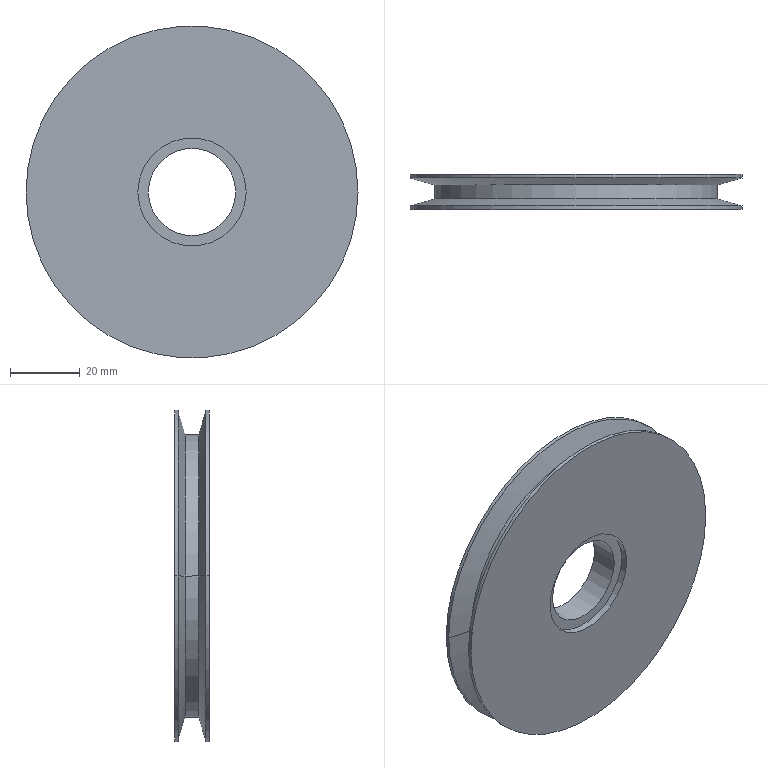Part | STEP file | BCC3 H16_2 | 1 solid | 17 faces | box 95 x 10 x 95 mm | volume 53732 mm3 | cylinder 10 | cone 4 | plane 3 | commonest cylinder face diameters 95 x4 25 x2 31 x2 81 x2
STEP:
#1=CARTESIAN_POINT('',(0.,0.,0.));
#2=DIRECTION('',(0.,0.,1.));
#3=DIRECTION('',(1.,0.,0.));
#4=AXIS2_PLACEMENT_3D('',#1,#2,#3);
#5=CARTESIAN_POINT('',(15.5,2.,0.));
#6=VERTEX_POINT('',#5);
#7=CARTESIAN_POINT('',(15.5,0.,0.));
#8=VERTEX_POINT('',#7);
#9=CARTESIAN_POINT('',(15.5,2.,0.));
#10=DIRECTION('',(0.,-1.,0.));
#11=VECTOR('',#10,1.);
#12=LINE('',#9,#11);
#13=CARTESIAN_POINT('',(0.,2.,0.));
#14=DIRECTION('',(0.,-1.,0.));
#15=DIRECTION('',(1.,0.,0.));
#16=AXIS2_PLACEMENT_3D('',#13,#14,#15);
#17=CYLINDRICAL_SURFACE('',#16,15.5);
#18=CARTESIAN_POINT('',(6.283,0.));
#19=DIRECTION('',(0.,1.));
#20=VECTOR('',#19,1.);
#21=LINE('',#18,#20);
#22=(GEOMETRIC_REPRESENTATION_CONTEXT(2)PARAMETRIC_REPRESENTATION_CONTEXT()REPRESENTATION_CONTEXT('',''));
#23=DEFINITIONAL_REPRESENTATION('',(#21),#22);
#24=PCURVE('',#17,#23);
#25=CARTESIAN_POINT('',(0.,2.,0.));
#26=DIRECTION('',(0.,-1.,0.));
#27=DIRECTION('',(1.,0.,0.));
#28=AXIS2_PLACEMENT_3D('',#25,#26,#27);
#29=CYLINDRICAL_SURFACE('',#28,15.5);
#30=CARTESIAN_POINT('',(0.,0.));
#31=DIRECTION('',(0.,1.));
#32=VECTOR('',#31,1.);
#33=LINE('',#30,#32);
#34=(GEOMETRIC_REPRESENTATION_CONTEXT(2)PARAMETRIC_REPRESENTATION_CONTEXT()REPRESENTATION_CONTEXT('',''));
#35=DEFINITIONAL_REPRESENTATION('',(#33),#34);
#36=PCURVE('',#29,#35);
#37=SURFACE_CURVE('',#12,(#24,#36),.PCURVE_S1.);
#38=EDGE_CURVE('',#6,#8,#37,.T.);
#39=ORIENTED_EDGE('',*,*,#38,.T.);
#40=CARTESIAN_POINT('',(-15.5,0.,0.));
#41=VERTEX_POINT('',#40);
#42=CARTESIAN_POINT('',(0.,0.,0.));
#43=DIRECTION('',(0.,1.,0.));
#44=DIRECTION('',(-1.,0.,0.));
#45=AXIS2_PLACEMENT_3D('',#42,#43,#44);
#46=CIRCLE('',#45,15.5);
#47=CARTESIAN_POINT('',(9.425,2.));
#48=DIRECTION('',(-1.,0.));
#49=VECTOR('',#48,1.);
#50=LINE('',#47,#49);
#51=(GEOMETRIC_REPRESENTATION_CONTEXT(2)PARAMETRIC_REPRESENTATION_CONTEXT()REPRESENTATION_CONTEXT('',''));
#52=DEFINITIONAL_REPRESENTATION('',(#50),#51);
#53=PCURVE('',#17,#52);
#54=CARTESIAN_POINT('',(47.5,0.,0.));
#55=DIRECTION('',(0.,-1.,0.));
#56=DIRECTION('',(1.,0.,0.));
#57=AXIS2_PLACEMENT_3D('',#54,#55,#56);
#58=PLANE('',#57);
#59=CARTESIAN_POINT('',(-63.,0.));
#60=CARTESIAN_POINT('',(-63.,26.847));
#61=CARTESIAN_POINT('',(-39.75,13.423));
#62=CARTESIAN_POINT('',(-16.5,0.));
#63=CARTESIAN_POINT('',(-39.75,-13.423));
#64=CARTESIAN_POINT('',(-63.,-26.847));
#65=CARTESIAN_POINT('',(-63.,0.));
#66=(BOUNDED_CURVE()B_SPLINE_CURVE(2,(#59,#60,#61,#62,#63,#64,#65),.UNSPECIFIED.,.T.,.F.)B_SPLINE_CURVE_WITH_KNOTS((1,2,2,2,2,1),(-2.094,0.,2.094,4.189,6.283,8.378),.UNSPECIFIED.)CURVE()GEOMETRIC_REPRESENTATION_ITEM()RATIONAL_B_SPLINE_CURVE((1.,0.5,1.,0.5,1.,0.5,1.))REPRESENTATION_ITEM(''));
#67=(GEOMETRIC_REPRESENTATION_CONTEXT(2)PARAMETRIC_REPRESENTATION_CONTEXT()REPRESENTATION_CONTEXT('',''));
#68=DEFINITIONAL_REPRESENTATION('',(#66),#67);
#69=PCURVE('',#58,#68);
#70=SURFACE_CURVE('',#46,(#53,#69),.PCURVE_S1.);
#71=EDGE_CURVE('',#8,#41,#70,.T.);
#72=ORIENTED_EDGE('',*,*,#71,.T.);
#73=CARTESIAN_POINT('',(-15.5,2.,0.));
#74=VERTEX_POINT('',#73);
#75=CARTESIAN_POINT('',(-15.5,2.,0.));
#76=DIRECTION('',(0.,-1.,0.));
#77=VECTOR('',#76,1.);
#78=LINE('',#75,#77);
#79=CARTESIAN_POINT('',(3.142,0.));
#80=DIRECTION('',(0.,1.));
#81=VECTOR('',#80,1.);
#82=LINE('',#79,#81);
#83=(GEOMETRIC_REPRESENTATION_CONTEXT(2)PARAMETRIC_REPRESENTATION_CONTEXT()REPRESENTATION_CONTEXT('',''));
#84=DEFINITIONAL_REPRESENTATION('',(#82),#83);
#85=PCURVE('',#17,#84);
#86=CARTESIAN_POINT('',(3.142,0.));
#87=DIRECTION('',(0.,1.));
#88=VECTOR('',#87,1.);
#89=LINE('',#86,#88);
#90=(GEOMETRIC_REPRESENTATION_CONTEXT(2)PARAMETRIC_REPRESENTATION_CONTEXT()REPRESENTATION_CONTEXT('',''));
#91=DEFINITIONAL_REPRESENTATION('',(#89),#90);
#92=PCURVE('',#29,#91);
#93=SURFACE_CURVE('',#78,(#85,#92),.PCURVE_S1.);
#94=EDGE_CURVE('',#74,#41,#93,.T.);
#95=ORIENTED_EDGE('',*,*,#94,.F.);
#96=CARTESIAN_POINT('',(0.,2.,0.));
#97=DIRECTION('',(0.,1.,0.));
#98=DIRECTION('',(-1.,0.,0.));
#99=AXIS2_PLACEMENT_3D('',#96,#97,#98);
#100=CIRCLE('',#99,15.5);
#101=CARTESIAN_POINT('',(9.425,0.));
#102=DIRECTION('',(-1.,0.));
#103=VECTOR('',#102,1.);
#104=LINE('',#101,#103);
#105=(GEOMETRIC_REPRESENTATION_CONTEXT(2)PARAMETRIC_REPRESENTATION_CONTEXT()REPRESENTATION_CONTEXT('',''));
#106=DEFINITIONAL_REPRESENTATION('',(#104),#105);
#107=PCURVE('',#17,#106);
#108=CARTESIAN_POINT('',(0.,2.,0.));
#109=DIRECTION('',(0.,1.,0.));
#110=DIRECTION('',(-1.,0.,0.));
#111=AXIS2_PLACEMENT_3D('',#108,#109,#110);
#112=PLANE('',#111);
#113=CARTESIAN_POINT('',(0.,0.));
#114=DIRECTION('',(1.,0.));
#115=AXIS2_PLACEMENT_2D('',#113,#114);
#116=CIRCLE('',#115,15.5);
#117=(GEOMETRIC_REPRESENTATION_CONTEXT(2)PARAMETRIC_REPRESENTATION_CONTEXT()REPRESENTATION_CONTEXT('',''));
#118=DEFINITIONAL_REPRESENTATION('',(#116),#117);
#119=PCURVE('',#112,#118);
#120=SURFACE_CURVE('',#100,(#107,#119),.PCURVE_S1.);
#121=EDGE_CURVE('',#6,#74,#120,.T.);
#122=ORIENTED_EDGE('',*,*,#121,.F.);
#123=EDGE_LOOP('',(#39,#72,#95,#122));
#124=FACE_BOUND('',#123,.F.);
#125=ADVANCED_FACE('',(#124),#17,.F.);
#126=CARTESIAN_POINT('',(12.5,10.,0.));
#127=VERTEX_POINT('',#126);
#128=CARTESIAN_POINT('',(12.5,2.,0.));
#129=VERTEX_POINT('',#128);
#130=CARTESIAN_POINT('',(12.5,0.,0.));
#131=DIRECTION('',(0.,-1.,0.));
#132=VECTOR('',#131,1.);
#133=LINE('',#130,#132);
#134=CARTESIAN_POINT('',(0.,0.,0.));
#135=DIRECTION('',(0.,-1.,0.));
#136=DIRECTION('',(1.,0.,0.));
#137=AXIS2_PLACEMENT_3D('',#134,#135,#136);
#138=CYLINDRICAL_SURFACE('',#137,12.5);
#139=CARTESIAN_POINT('',(6.283,0.));
#140=DIRECTION('',(0.,1.));
#141=VECTOR('',#140,1.);
#142=LINE('',#139,#141);
#143=(GEOMETRIC_REPRESENTATION_CONTEXT(2)PARAMETRIC_REPRESENTATION_CONTEXT()REPRESENTATION_CONTEXT('',''));
#144=DEFINITIONAL_REPRESENTATION('',(#142),#143);
#145=PCURVE('',#138,#144);
#146=CARTESIAN_POINT('',(0.,0.,0.));
#147=DIRECTION('',(0.,-1.,0.));
#148=DIRECTION('',(1.,0.,0.));
#149=AXIS2_PLACEMENT_3D('',#146,#147,#148);
#150=CYLINDRICAL_SURFACE('',#149,12.5);
#151=CARTESIAN_POINT('',(0.,0.));
#152=DIRECTION('',(0.,1.));
#153=VECTOR('',#152,1.);
#154=LINE('',#151,#153);
#155=(GEOMETRIC_REPRESENTATION_CONTEXT(2)PARAMETRIC_REPRESENTATION_CONTEXT()REPRESENTATION_CONTEXT('',''));
#156=DEFINITIONAL_REPRESENTATION('',(#154),#155);
#157=PCURVE('',#150,#156);
#158=SURFACE_CURVE('',#133,(#145,#157),.PCURVE_S1.);
#159=EDGE_CURVE('',#127,#129,#158,.T.);
#160=ORIENTED_EDGE('',*,*,#159,.T.);
#161=CARTESIAN_POINT('',(-12.5,2.,0.));
#162=VERTEX_POINT('',#161);
#163=CARTESIAN_POINT('',(0.,2.,0.));
#164=DIRECTION('',(0.,1.,0.));
#165=DIRECTION('',(-1.,0.,0.));
#166=AXIS2_PLACEMENT_3D('',#163,#164,#165);
#167=CIRCLE('',#166,12.5);
#168=CARTESIAN_POINT('',(9.425,-2.));
#169=DIRECTION('',(-1.,0.));
#170=VECTOR('',#169,1.);
#171=LINE('',#168,#170);
#172=(GEOMETRIC_REPRESENTATION_CONTEXT(2)PARAMETRIC_REPRESENTATION_CONTEXT()REPRESENTATION_CONTEXT('',''));
#173=DEFINITIONAL_REPRESENTATION('',(#171),#172);
#174=PCURVE('',#138,#173);
#175=CARTESIAN_POINT('',(0.,0.));
#176=DIRECTION('',(1.,0.));
#177=AXIS2_PLACEMENT_2D('',#175,#176);
#178=CIRCLE('',#177,12.5);
#179=(GEOMETRIC_REPRESENTATION_CONTEXT(2)PARAMETRIC_REPRESENTATION_CONTEXT()REPRESENTATION_CONTEXT('',''));
#180=DEFINITIONAL_REPRESENTATION('',(#178),#179);
#181=PCURVE('',#112,#180);
#182=SURFACE_CURVE('',#167,(#174,#181),.PCURVE_S1.);
#183=EDGE_CURVE('',#129,#162,#182,.T.);
#184=ORIENTED_EDGE('',*,*,#183,.T.);
#185=CARTESIAN_POINT('',(-12.5,10.,0.));
#186=VERTEX_POINT('',#185);
#187=CARTESIAN_POINT('',(-12.5,0.,0.));
#188=DIRECTION('',(0.,-1.,0.));
#189=VECTOR('',#188,1.);
#190=LINE('',#187,#189);
#191=CARTESIAN_POINT('',(3.142,0.));
#192=DIRECTION('',(0.,1.));
#193=VECTOR('',#192,1.);
#194=LINE('',#191,#193);
#195=(GEOMETRIC_REPRESENTATION_CONTEXT(2)PARAMETRIC_REPRESENTATION_CONTEXT()REPRESENTATION_CONTEXT('',''));
#196=DEFINITIONAL_REPRESENTATION('',(#194),#195);
#197=PCURVE('',#138,#196);
#198=CARTESIAN_POINT('',(3.142,0.));
#199=DIRECTION('',(0.,1.));
#200=VECTOR('',#199,1.);
#201=LINE('',#198,#200);
#202=(GEOMETRIC_REPRESENTATION_CONTEXT(2)PARAMETRIC_REPRESENTATION_CONTEXT()REPRESENTATION_CONTEXT('',''));
#203=DEFINITIONAL_REPRESENTATION('',(#201),#202);
#204=PCURVE('',#150,#203);
#205=SURFACE_CURVE('',#190,(#197,#204),.PCURVE_S1.);
#206=EDGE_CURVE('',#186,#162,#205,.T.);
#207=ORIENTED_EDGE('',*,*,#206,.F.);
#208=CARTESIAN_POINT('',(0.,10.,0.));
#209=DIRECTION('',(0.,-1.,0.));
#210=DIRECTION('',(1.,0.,0.));
#211=AXIS2_PLACEMENT_3D('',#208,#209,#210);
#212=CIRCLE('',#211,12.5);
#213=CARTESIAN_POINT('',(0.,-10.));
#214=DIRECTION('',(1.,0.));
#215=VECTOR('',#214,1.);
#216=LINE('',#213,#215);
#217=(GEOMETRIC_REPRESENTATION_CONTEXT(2)PARAMETRIC_REPRESENTATION_CONTEXT()REPRESENTATION_CONTEXT('',''));
#218=DEFINITIONAL_REPRESENTATION('',(#216),#217);
#219=PCURVE('',#138,#218);
#220=CARTESIAN_POINT('',(12.5,10.,0.));
#221=DIRECTION('',(0.,1.,0.));
#222=DIRECTION('',(-1.,0.,0.));
#223=AXIS2_PLACEMENT_3D('',#220,#221,#222);
#224=PLANE('',#223);
#225=CARTESIAN_POINT('',(0.,0.));
#226=CARTESIAN_POINT('',(0.,21.651));
#227=CARTESIAN_POINT('',(18.75,10.825));
#228=CARTESIAN_POINT('',(37.5,0.));
#229=CARTESIAN_POINT('',(18.75,-10.825));
#230=CARTESIAN_POINT('',(0.,-21.651));
#231=CARTESIAN_POINT('',(0.,0.));
#232=(BOUNDED_CURVE()B_SPLINE_CURVE(2,(#225,#226,#227,#228,#229,#230,#231),.UNSPECIFIED.,.T.,.F.)B_SPLINE_CURVE_WITH_KNOTS((1,2,2,2,2,1),(-2.094,0.,2.094,4.189,6.283,8.378),.UNSPECIFIED.)CURVE()GEOMETRIC_REPRESENTATION_ITEM()RATIONAL_B_SPLINE_CURVE((1.,0.5,1.,0.5,1.,0.5,1.))REPRESENTATION_ITEM(''));
#233=(GEOMETRIC_REPRESENTATION_CONTEXT(2)PARAMETRIC_REPRESENTATION_CONTEXT()REPRESENTATION_CONTEXT('',''));
#234=DEFINITIONAL_REPRESENTATION('',(#232),#233);
#235=PCURVE('',#224,#234);
#236=SURFACE_CURVE('',#212,(#219,#235),.PCURVE_S1.);
#237=EDGE_CURVE('',#186,#127,#236,.T.);
#238=ORIENTED_EDGE('',*,*,#237,.T.);
#239=EDGE_LOOP('',(#160,#184,#207,#238));
#240=FACE_BOUND('',#239,.F.);
#241=ADVANCED_FACE('',(#240),#138,.F.);
#242=CARTESIAN_POINT('',(47.5,1.,0.));
#243=VERTEX_POINT('',#242);
#244=CARTESIAN_POINT('',(-47.5,1.,0.));
#245=VERTEX_POINT('',#244);
#246=CARTESIAN_POINT('',(0.,1.,0.));
#247=DIRECTION('',(0.,-1.,0.));
#248=DIRECTION('',(1.,0.,0.));
#249=AXIS2_PLACEMENT_3D('',#246,#247,#248);
#250=CIRCLE('',#249,47.5);
#251=CARTESIAN_POINT('',(0.,0.,0.));
#252=DIRECTION('',(0.,-1.,0.));
#253=DIRECTION('',(1.,0.,0.));
#254=AXIS2_PLACEMENT_3D('',#251,#252,#253);
#255=CYLINDRICAL_SURFACE('',#254,47.5);
#256=CARTESIAN_POINT('',(0.,-1.));
#257=DIRECTION('',(1.,0.));
#258=VECTOR('',#257,1.);
#259=LINE('',#256,#258);
#260=(GEOMETRIC_REPRESENTATION_CONTEXT(2)PARAMETRIC_REPRESENTATION_CONTEXT()REPRESENTATION_CONTEXT('',''));
#261=DEFINITIONAL_REPRESENTATION('',(#259),#260);
#262=PCURVE('',#255,#261);
#263=CARTESIAN_POINT('',(0.,1.,0.));
#264=DIRECTION('',(0.,-1.,0.));
#265=DIRECTION('',(1.,0.,0.));
#266=AXIS2_PLACEMENT_3D('',#263,#264,#265);
#267=CONICAL_SURFACE('',#266,47.5,1.292);
#268=CARTESIAN_POINT('',(0.,0.));
#269=DIRECTION('',(1.,0.));
#270=VECTOR('',#269,1.);
#271=LINE('',#268,#270);
#272=(GEOMETRIC_REPRESENTATION_CONTEXT(2)PARAMETRIC_REPRESENTATION_CONTEXT()REPRESENTATION_CONTEXT('',''));
#273=DEFINITIONAL_REPRESENTATION('',(#271),#272);
#274=PCURVE('',#267,#273);
#275=SURFACE_CURVE('',#250,(#262,#274),.PCURVE_S1.);
#276=EDGE_CURVE('',#243,#245,#275,.T.);
#277=ORIENTED_EDGE('',*,*,#276,.T.);
#278=CARTESIAN_POINT('',(-47.5,0.,0.));
#279=VERTEX_POINT('',#278);
#280=CARTESIAN_POINT('',(-47.5,0.,0.));
#281=DIRECTION('',(0.,-1.,0.));
#282=VECTOR('',#281,1.);
#283=LINE('',#280,#282);
#284=CARTESIAN_POINT('',(3.142,0.));
#285=DIRECTION('',(0.,1.));
#286=VECTOR('',#285,1.);
#287=LINE('',#284,#286);
#288=(GEOMETRIC_REPRESENTATION_CONTEXT(2)PARAMETRIC_REPRESENTATION_CONTEXT()REPRESENTATION_CONTEXT('',''));
#289=DEFINITIONAL_REPRESENTATION('',(#287),#288);
#290=PCURVE('',#255,#289);
#291=CARTESIAN_POINT('',(0.,0.,0.));
#292=DIRECTION('',(0.,-1.,0.));
#293=DIRECTION('',(1.,0.,0.));
#294=AXIS2_PLACEMENT_3D('',#291,#292,#293);
#295=CYLINDRICAL_SURFACE('',#294,47.5);
#296=CARTESIAN_POINT('',(3.142,0.));
#297=DIRECTION('',(0.,1.));
#298=VECTOR('',#297,1.);
#299=LINE('',#296,#298);
#300=(GEOMETRIC_REPRESENTATION_CONTEXT(2)PARAMETRIC_REPRESENTATION_CONTEXT()REPRESENTATION_CONTEXT('',''));
#301=DEFINITIONAL_REPRESENTATION('',(#299),#300);
#302=PCURVE('',#295,#301);
#303=SURFACE_CURVE('',#283,(#290,#302),.PCURVE_S1.);
#304=EDGE_CURVE('',#245,#279,#303,.T.);
#305=ORIENTED_EDGE('',*,*,#304,.T.);
#306=CARTESIAN_POINT('',(47.5,0.,0.));
#307=VERTEX_POINT('',#306);
#308=CARTESIAN_POINT('',(0.,0.,0.));
#309=DIRECTION('',(0.,-1.,0.));
#310=DIRECTION('',(1.,0.,0.));
#311=AXIS2_PLACEMENT_3D('',#308,#309,#310);
#312=CIRCLE('',#311,47.5);
#313=CARTESIAN_POINT('',(0.,0.));
#314=DIRECTION('',(1.,0.));
#315=VECTOR('',#314,1.);
#316=LINE('',#313,#315);
#317=(GEOMETRIC_REPRESENTATION_CONTEXT(2)PARAMETRIC_REPRESENTATION_CONTEXT()REPRESENTATION_CONTEXT('',''));
#318=DEFINITIONAL_REPRESENTATION('',(#316),#317);
#319=PCURVE('',#255,#318);
#320=CARTESIAN_POINT('',(-47.5,0.));
#321=DIRECTION('',(1.,0.));
#322=AXIS2_PLACEMENT_2D('',#320,#321);
#323=CIRCLE('',#322,47.5);
#324=(GEOMETRIC_REPRESENTATION_CONTEXT(2)PARAMETRIC_REPRESENTATION_CONTEXT()REPRESENTATION_CONTEXT('',''));
#325=DEFINITIONAL_REPRESENTATION('',(#323),#324);
#326=PCURVE('',#58,#325);
#327=SURFACE_CURVE('',#312,(#319,#326),.PCURVE_S1.);
#328=EDGE_CURVE('',#307,#279,#327,.T.);
#329=ORIENTED_EDGE('',*,*,#328,.F.);
#330=CARTESIAN_POINT('',(47.5,0.,0.));
#331=DIRECTION('',(0.,-1.,0.));
#332=VECTOR('',#331,1.);
#333=LINE('',#330,#332);
#334=CARTESIAN_POINT('',(0.,0.));
#335=DIRECTION('',(0.,1.));
#336=VECTOR('',#335,1.);
#337=LINE('',#334,#336);
#338=(GEOMETRIC_REPRESENTATION_CONTEXT(2)PARAMETRIC_REPRESENTATION_CONTEXT()REPRESENTATION_CONTEXT('',''));
#339=DEFINITIONAL_REPRESENTATION('',(#337),#338);
#340=PCURVE('',#255,#339);
#341=CARTESIAN_POINT('',(6.283,0.));
#342=DIRECTION('',(0.,1.));
#343=VECTOR('',#342,1.);
#344=LINE('',#341,#343);
#345=(GEOMETRIC_REPRESENTATION_CONTEXT(2)PARAMETRIC_REPRESENTATION_CONTEXT()REPRESENTATION_CONTEXT('',''));
#346=DEFINITIONAL_REPRESENTATION('',(#344),#345);
#347=PCURVE('',#295,#346);
#348=SURFACE_CURVE('',#333,(#340,#347),.PCURVE_S1.);
#349=EDGE_CURVE('',#243,#307,#348,.T.);
#350=ORIENTED_EDGE('',*,*,#349,.F.);
#351=EDGE_LOOP('',(#277,#305,#329,#350));
#352=FACE_BOUND('',#351,.T.);
#353=ADVANCED_FACE('',(#352),#255,.T.);
#354=CARTESIAN_POINT('',(40.5,3.,0.));
#355=VERTEX_POINT('',#354);
#356=CARTESIAN_POINT('',(-40.5,3.,0.));
#357=VERTEX_POINT('',#356);
#358=CARTESIAN_POINT('',(0.,3.,0.));
#359=DIRECTION('',(0.,-1.,0.));
#360=DIRECTION('',(1.,0.,0.));
#361=AXIS2_PLACEMENT_3D('',#358,#359,#360);
#362=CIRCLE('',#361,40.5);
#363=CARTESIAN_POINT('',(0.,-2.));
#364=DIRECTION('',(1.,0.));
#365=VECTOR('',#364,1.);
#366=LINE('',#363,#365);
#367=(GEOMETRIC_REPRESENTATION_CONTEXT(2)PARAMETRIC_REPRESENTATION_CONTEXT()REPRESENTATION_CONTEXT('',''));
#368=DEFINITIONAL_REPRESENTATION('',(#366),#367);
#369=PCURVE('',#267,#368);
#370=CARTESIAN_POINT('',(0.,0.,0.));
#371=DIRECTION('',(0.,-1.,0.));
#372=DIRECTION('',(1.,0.,0.));
#373=AXIS2_PLACEMENT_3D('',#370,#371,#372);
#374=CYLINDRICAL_SURFACE('',#373,40.5);
#375=CARTESIAN_POINT('',(0.,-3.));
#376=DIRECTION('',(1.,0.));
#377=VECTOR('',#376,1.);
#378=LINE('',#375,#377);
#379=(GEOMETRIC_REPRESENTATION_CONTEXT(2)PARAMETRIC_REPRESENTATION_CONTEXT()REPRESENTATION_CONTEXT('',''));
#380=DEFINITIONAL_REPRESENTATION('',(#378),#379);
#381=PCURVE('',#374,#380);
#382=SURFACE_CURVE('',#362,(#369,#381),.PCURVE_S1.);
#383=EDGE_CURVE('',#355,#357,#382,.T.);
#384=ORIENTED_EDGE('',*,*,#383,.T.);
#385=CARTESIAN_POINT('',(-47.5,1.,0.));
#386=DIRECTION('',(-0.9615,-0.2747,0.));
#387=VECTOR('',#386,1.);
#388=LINE('',#385,#387);
#389=CARTESIAN_POINT('',(3.142,0.));
#390=DIRECTION('',(0.,1.));
#391=VECTOR('',#390,1.);
#392=LINE('',#389,#391);
#393=(GEOMETRIC_REPRESENTATION_CONTEXT(2)PARAMETRIC_REPRESENTATION_CONTEXT()REPRESENTATION_CONTEXT('',''));
#394=DEFINITIONAL_REPRESENTATION('',(#392),#393);
#395=PCURVE('',#267,#394);
#396=CARTESIAN_POINT('',(0.,1.,0.));
#397=DIRECTION('',(0.,-1.,0.));
#398=DIRECTION('',(1.,0.,0.));
#399=AXIS2_PLACEMENT_3D('',#396,#397,#398);
#400=CONICAL_SURFACE('',#399,47.5,1.292);
#401=CARTESIAN_POINT('',(3.142,0.));
#402=DIRECTION('',(0.,1.));
#403=VECTOR('',#402,1.);
#404=LINE('',#401,#403);
#405=(GEOMETRIC_REPRESENTATION_CONTEXT(2)PARAMETRIC_REPRESENTATION_CONTEXT()REPRESENTATION_CONTEXT('',''));
#406=DEFINITIONAL_REPRESENTATION('',(#404),#405);
#407=PCURVE('',#400,#406);
#408=SURFACE_CURVE('',#388,(#395,#407),.PCURVE_S1.);
#409=EDGE_CURVE('',#357,#245,#408,.T.);
#410=ORIENTED_EDGE('',*,*,#409,.T.);
#411=ORIENTED_EDGE('',*,*,#276,.F.);
#412=CARTESIAN_POINT('',(47.5,1.,0.));
#413=DIRECTION('',(0.9615,-0.2747,0.));
#414=VECTOR('',#413,1.);
#415=LINE('',#412,#414);
#416=CARTESIAN_POINT('',(0.,0.));
#417=DIRECTION('',(0.,1.));
#418=VECTOR('',#417,1.);
#419=LINE('',#416,#418);
#420=(GEOMETRIC_REPRESENTATION_CONTEXT(2)PARAMETRIC_REPRESENTATION_CONTEXT()REPRESENTATION_CONTEXT('',''));
#421=DEFINITIONAL_REPRESENTATION('',(#419),#420);
#422=PCURVE('',#267,#421);
#423=CARTESIAN_POINT('',(6.283,0.));
#424=DIRECTION('',(0.,1.));
#425=VECTOR('',#424,1.);
#426=LINE('',#423,#425);
#427=(GEOMETRIC_REPRESENTATION_CONTEXT(2)PARAMETRIC_REPRESENTATION_CONTEXT()REPRESENTATION_CONTEXT('',''));
#428=DEFINITIONAL_REPRESENTATION('',(#426),#427);
#429=PCURVE('',#400,#428);
#430=SURFACE_CURVE('',#415,(#422,#429),.PCURVE_S1.);
#431=EDGE_CURVE('',#355,#243,#430,.T.);
#432=ORIENTED_EDGE('',*,*,#431,.F.);
#433=EDGE_LOOP('',(#384,#410,#411,#432));
#434=FACE_BOUND('',#433,.T.);
#435=ADVANCED_FACE('',(#434),#267,.T.);
#436=CARTESIAN_POINT('',(40.5,7.,0.));
#437=VERTEX_POINT('',#436);
#438=CARTESIAN_POINT('',(-40.5,7.,0.));
#439=VERTEX_POINT('',#438);
#440=CARTESIAN_POINT('',(0.,7.,0.));
#441=DIRECTION('',(0.,-1.,0.));
#442=DIRECTION('',(1.,0.,0.));
#443=AXIS2_PLACEMENT_3D('',#440,#441,#442);
#444=CIRCLE('',#443,40.5);
#445=CARTESIAN_POINT('',(0.,-7.));
#446=DIRECTION('',(1.,0.));
#447=VECTOR('',#446,1.);
#448=LINE('',#445,#447);
#449=(GEOMETRIC_REPRESENTATION_CONTEXT(2)PARAMETRIC_REPRESENTATION_CONTEXT()REPRESENTATION_CONTEXT('',''));
#450=DEFINITIONAL_REPRESENTATION('',(#448),#449);
#451=PCURVE('',#374,#450);
#452=CARTESIAN_POINT('',(0.,7.,0.));
#453=DIRECTION('',(0.,1.,0.));
#454=DIRECTION('',(-1.,0.,0.));
#455=AXIS2_PLACEMENT_3D('',#452,#453,#454);
#456=CONICAL_SURFACE('',#455,40.5,1.292);
#457=CARTESIAN_POINT('',(3.142,0.));
#458=DIRECTION('',(-1.,0.));
#459=VECTOR('',#458,1.);
#460=LINE('',#457,#459);
#461=(GEOMETRIC_REPRESENTATION_CONTEXT(2)PARAMETRIC_REPRESENTATION_CONTEXT()REPRESENTATION_CONTEXT('',''));
#462=DEFINITIONAL_REPRESENTATION('',(#460),#461);
#463=PCURVE('',#456,#462);
#464=SURFACE_CURVE('',#444,(#451,#463),.PCURVE_S1.);
#465=EDGE_CURVE('',#437,#439,#464,.T.);
#466=ORIENTED_EDGE('',*,*,#465,.T.);
#467=CARTESIAN_POINT('',(-40.5,0.,0.));
#468=DIRECTION('',(0.,-1.,0.));
#469=VECTOR('',#468,1.);
#470=LINE('',#467,#469);
#471=CARTESIAN_POINT('',(3.142,0.));
#472=DIRECTION('',(0.,1.));
#473=VECTOR('',#472,1.);
#474=LINE('',#471,#473);
#475=(GEOMETRIC_REPRESENTATION_CONTEXT(2)PARAMETRIC_REPRESENTATION_CONTEXT()REPRESENTATION_CONTEXT('',''));
#476=DEFINITIONAL_REPRESENTATION('',(#474),#475);
#477=PCURVE('',#374,#476);
#478=CARTESIAN_POINT('',(0.,0.,0.));
#479=DIRECTION('',(0.,-1.,0.));
#480=DIRECTION('',(1.,0.,0.));
#481=AXIS2_PLACEMENT_3D('',#478,#479,#480);
#482=CYLINDRICAL_SURFACE('',#481,40.5);
#483=CARTESIAN_POINT('',(3.142,0.));
#484=DIRECTION('',(0.,1.));
#485=VECTOR('',#484,1.);
#486=LINE('',#483,#485);
#487=(GEOMETRIC_REPRESENTATION_CONTEXT(2)PARAMETRIC_REPRESENTATION_CONTEXT()REPRESENTATION_CONTEXT('',''));
#488=DEFINITIONAL_REPRESENTATION('',(#486),#487);
#489=PCURVE('',#482,#488);
#490=SURFACE_CURVE('',#470,(#477,#489),.PCURVE_S1.);
#491=EDGE_CURVE('',#439,#357,#490,.T.);
#492=ORIENTED_EDGE('',*,*,#491,.T.);
#493=ORIENTED_EDGE('',*,*,#383,.F.);
#494=CARTESIAN_POINT('',(40.5,0.,0.));
#495=DIRECTION('',(0.,-1.,0.));
#496=VECTOR('',#495,1.);
#497=LINE('',#494,#496);
#498=CARTESIAN_POINT('',(0.,0.));
#499=DIRECTION('',(0.,1.));
#500=VECTOR('',#499,1.);
#501=LINE('',#498,#500);
#502=(GEOMETRIC_REPRESENTATION_CONTEXT(2)PARAMETRIC_REPRESENTATION_CONTEXT()REPRESENTATION_CONTEXT('',''));
#503=DEFINITIONAL_REPRESENTATION('',(#501),#502);
#504=PCURVE('',#374,#503);
#505=CARTESIAN_POINT('',(6.283,0.));
#506=DIRECTION('',(0.,1.));
#507=VECTOR('',#506,1.);
#508=LINE('',#505,#507);
#509=(GEOMETRIC_REPRESENTATION_CONTEXT(2)PARAMETRIC_REPRESENTATION_CONTEXT()REPRESENTATION_CONTEXT('',''));
#510=DEFINITIONAL_REPRESENTATION('',(#508),#509);
#511=PCURVE('',#482,#510);
#512=SURFACE_CURVE('',#497,(#504,#511),.PCURVE_S1.);
#513=EDGE_CURVE('',#437,#355,#512,.T.);
#514=ORIENTED_EDGE('',*,*,#513,.F.);
#515=EDGE_LOOP('',(#466,#492,#493,#514));
#516=FACE_BOUND('',#515,.T.);
#517=ADVANCED_FACE('',(#516),#374,.T.);
#518=ORIENTED_EDGE('',*,*,#465,.F.);
#519=CARTESIAN_POINT('',(47.5,9.,0.));
#520=VERTEX_POINT('',#519);
#521=CARTESIAN_POINT('',(40.5,7.,0.));
#522=DIRECTION('',(0.9615,0.2747,0.));
#523=VECTOR('',#522,1.);
#524=LINE('',#521,#523);
#525=CARTESIAN_POINT('',(3.142,0.));
#526=DIRECTION('',(0.,1.));
#527=VECTOR('',#526,1.);
#528=LINE('',#525,#527);
#529=(GEOMETRIC_REPRESENTATION_CONTEXT(2)PARAMETRIC_REPRESENTATION_CONTEXT()REPRESENTATION_CONTEXT('',''));
#530=DEFINITIONAL_REPRESENTATION('',(#528),#529);
#531=PCURVE('',#456,#530);
#532=CARTESIAN_POINT('',(0.,7.,0.));
#533=DIRECTION('',(0.,1.,0.));
#534=DIRECTION('',(-1.,0.,0.));
#535=AXIS2_PLACEMENT_3D('',#532,#533,#534);
#536=CONICAL_SURFACE('',#535,40.5,1.292);
#537=CARTESIAN_POINT('',(3.142,0.));
#538=DIRECTION('',(0.,1.));
#539=VECTOR('',#538,1.);
#540=LINE('',#537,#539);
#541=(GEOMETRIC_REPRESENTATION_CONTEXT(2)PARAMETRIC_REPRESENTATION_CONTEXT()REPRESENTATION_CONTEXT('',''));
#542=DEFINITIONAL_REPRESENTATION('',(#540),#541);
#543=PCURVE('',#536,#542);
#544=SURFACE_CURVE('',#524,(#531,#543),.PCURVE_S1.);
#545=EDGE_CURVE('',#437,#520,#544,.T.);
#546=ORIENTED_EDGE('',*,*,#545,.T.);
#547=CARTESIAN_POINT('',(-47.5,9.,0.));
#548=VERTEX_POINT('',#547);
#549=CARTESIAN_POINT('',(0.,9.,0.));
#550=DIRECTION('',(0.,-1.,0.));
#551=DIRECTION('',(1.,0.,0.));
#552=AXIS2_PLACEMENT_3D('',#549,#550,#551);
#553=CIRCLE('',#552,47.5);
#554=CARTESIAN_POINT('',(3.142,2.));
#555=DIRECTION('',(-1.,0.));
#556=VECTOR('',#555,1.);
#557=LINE('',#554,#556);
#558=(GEOMETRIC_REPRESENTATION_CONTEXT(2)PARAMETRIC_REPRESENTATION_CONTEXT()REPRESENTATION_CONTEXT('',''));
#559=DEFINITIONAL_REPRESENTATION('',(#557),#558);
#560=PCURVE('',#456,#559);
#561=CARTESIAN_POINT('',(0.,0.,0.));
#562=DIRECTION('',(0.,-1.,0.));
#563=DIRECTION('',(1.,0.,0.));
#564=AXIS2_PLACEMENT_3D('',#561,#562,#563);
#565=CYLINDRICAL_SURFACE('',#564,47.5);
#566=CARTESIAN_POINT('',(0.,-9.));
#567=DIRECTION('',(1.,0.));
#568=VECTOR('',#567,1.);
#569=LINE('',#566,#568);
#570=(GEOMETRIC_REPRESENTATION_CONTEXT(2)PARAMETRIC_REPRESENTATION_CONTEXT()REPRESENTATION_CONTEXT('',''));
#571=DEFINITIONAL_REPRESENTATION('',(#569),#570);
#572=PCURVE('',#565,#571);
#573=SURFACE_CURVE('',#553,(#560,#572),.PCURVE_S1.);
#574=EDGE_CURVE('',#520,#548,#573,.T.);
#575=ORIENTED_EDGE('',*,*,#574,.T.);
#576=CARTESIAN_POINT('',(-40.5,7.,0.));
#577=DIRECTION('',(-0.9615,0.2747,0.));
#578=VECTOR('',#577,1.);
#579=LINE('',#576,#578);
#580=CARTESIAN_POINT('',(0.,0.));
#581=DIRECTION('',(0.,1.));
#582=VECTOR('',#581,1.);
#583=LINE('',#580,#582);
#584=(GEOMETRIC_REPRESENTATION_CONTEXT(2)PARAMETRIC_REPRESENTATION_CONTEXT()REPRESENTATION_CONTEXT('',''));
#585=DEFINITIONAL_REPRESENTATION('',(#583),#584);
#586=PCURVE('',#456,#585);
#587=CARTESIAN_POINT('',(6.283,0.));
#588=DIRECTION('',(0.,1.));
#589=VECTOR('',#588,1.);
#590=LINE('',#587,#589);
#591=(GEOMETRIC_REPRESENTATION_CONTEXT(2)PARAMETRIC_REPRESENTATION_CONTEXT()REPRESENTATION_CONTEXT('',''));
#592=DEFINITIONAL_REPRESENTATION('',(#590),#591);
#593=PCURVE('',#536,#592);
#594=SURFACE_CURVE('',#579,(#586,#593),.PCURVE_S1.);
#595=EDGE_CURVE('',#439,#548,#594,.T.);
#596=ORIENTED_EDGE('',*,*,#595,.F.);
#597=EDGE_LOOP('',(#518,#546,#575,#596));
#598=FACE_BOUND('',#597,.T.);
#599=ADVANCED_FACE('',(#598),#456,.T.);
#600=CARTESIAN_POINT('',(47.5,10.,0.));
#601=VERTEX_POINT('',#600);
#602=CARTESIAN_POINT('',(-47.5,10.,0.));
#603=VERTEX_POINT('',#602);
#604=CARTESIAN_POINT('',(0.,10.,0.));
#605=DIRECTION('',(0.,-1.,0.));
#606=DIRECTION('',(1.,0.,0.));
#607=AXIS2_PLACEMENT_3D('',#604,#605,#606);
#608=CIRCLE('',#607,47.5);
#609=CARTESIAN_POINT('',(0.,-10.));
#610=DIRECTION('',(1.,0.));
#611=VECTOR('',#610,1.);
#612=LINE('',#609,#611);
#613=(GEOMETRIC_REPRESENTATION_CONTEXT(2)PARAMETRIC_REPRESENTATION_CONTEXT()REPRESENTATION_CONTEXT('',''));
#614=DEFINITIONAL_REPRESENTATION('',(#612),#613);
#615=PCURVE('',#565,#614);
#616=CARTESIAN_POINT('',(-35.,0.));
#617=CARTESIAN_POINT('',(-35.,82.272));
#618=CARTESIAN_POINT('',(36.25,41.136));
#619=CARTESIAN_POINT('',(107.5,0.));
#620=CARTESIAN_POINT('',(36.25,-41.136));
#621=CARTESIAN_POINT('',(-35.,-82.272));
#622=CARTESIAN_POINT('',(-35.,0.));
#623=(BOUNDED_CURVE()B_SPLINE_CURVE(2,(#616,#617,#618,#619,#620,#621,#622),.UNSPECIFIED.,.T.,.F.)B_SPLINE_CURVE_WITH_KNOTS((1,2,2,2,2,1),(-2.094,0.,2.094,4.189,6.283,8.378),.UNSPECIFIED.)CURVE()GEOMETRIC_REPRESENTATION_ITEM()RATIONAL_B_SPLINE_CURVE((1.,0.5,1.,0.5,1.,0.5,1.))REPRESENTATION_ITEM(''));
#624=(GEOMETRIC_REPRESENTATION_CONTEXT(2)PARAMETRIC_REPRESENTATION_CONTEXT()REPRESENTATION_CONTEXT('',''));
#625=DEFINITIONAL_REPRESENTATION('',(#623),#624);
#626=PCURVE('',#224,#625);
#627=SURFACE_CURVE('',#608,(#615,#626),.PCURVE_S1.);
#628=EDGE_CURVE('',#601,#603,#627,.T.);
#629=ORIENTED_EDGE('',*,*,#628,.T.);
#630=CARTESIAN_POINT('',(-47.5,0.,0.));
#631=DIRECTION('',(0.,-1.,0.));
#632=VECTOR('',#631,1.);
#633=LINE('',#630,#632);
#634=CARTESIAN_POINT('',(3.142,0.));
#635=DIRECTION('',(0.,1.));
#636=VECTOR('',#635,1.);
#637=LINE('',#634,#636);
#638=(GEOMETRIC_REPRESENTATION_CONTEXT(2)PARAMETRIC_REPRESENTATION_CONTEXT()REPRESENTATION_CONTEXT('',''));
#639=DEFINITIONAL_REPRESENTATION('',(#637),#638);
#640=PCURVE('',#565,#639);
#641=CARTESIAN_POINT('',(0.,0.,0.));
#642=DIRECTION('',(0.,-1.,0.));
#643=DIRECTION('',(1.,0.,0.));
#644=AXIS2_PLACEMENT_3D('',#641,#642,#643);
#645=CYLINDRICAL_SURFACE('',#644,47.5);
#646=CARTESIAN_POINT('',(3.142,0.));
#647=DIRECTION('',(0.,1.));
#648=VECTOR('',#647,1.);
#649=LINE('',#646,#648);
#650=(GEOMETRIC_REPRESENTATION_CONTEXT(2)PARAMETRIC_REPRESENTATION_CONTEXT()REPRESENTATION_CONTEXT('',''));
#651=DEFINITIONAL_REPRESENTATION('',(#649),#650);
#652=PCURVE('',#645,#651);
#653=SURFACE_CURVE('',#633,(#640,#652),.PCURVE_S1.);
#654=EDGE_CURVE('',#603,#548,#653,.T.);
#655=ORIENTED_EDGE('',*,*,#654,.T.);
#656=ORIENTED_EDGE('',*,*,#574,.F.);
#657=CARTESIAN_POINT('',(47.5,0.,0.));
#658=DIRECTION('',(0.,-1.,0.));
#659=VECTOR('',#658,1.);
#660=LINE('',#657,#659);
#661=CARTESIAN_POINT('',(0.,0.));
#662=DIRECTION('',(0.,1.));
#663=VECTOR('',#662,1.);
#664=LINE('',#661,#663);
#665=(GEOMETRIC_REPRESENTATION_CONTEXT(2)PARAMETRIC_REPRESENTATION_CONTEXT()REPRESENTATION_CONTEXT('',''));
#666=DEFINITIONAL_REPRESENTATION('',(#664),#665);
#667=PCURVE('',#565,#666);
#668=CARTESIAN_POINT('',(6.283,0.));
#669=DIRECTION('',(0.,1.));
#670=VECTOR('',#669,1.);
#671=LINE('',#668,#670);
#672=(GEOMETRIC_REPRESENTATION_CONTEXT(2)PARAMETRIC_REPRESENTATION_CONTEXT()REPRESENTATION_CONTEXT('',''));
#673=DEFINITIONAL_REPRESENTATION('',(#671),#672);
#674=PCURVE('',#645,#673);
#675=SURFACE_CURVE('',#660,(#667,#674),.PCURVE_S1.);
#676=EDGE_CURVE('',#601,#520,#675,.T.);
#677=ORIENTED_EDGE('',*,*,#676,.F.);
#678=EDGE_LOOP('',(#629,#655,#656,#677));
#679=FACE_BOUND('',#678,.T.);
#680=ADVANCED_FACE('',(#679),#565,.T.);
#681=ORIENTED_EDGE('',*,*,#328,.T.);
#682=CARTESIAN_POINT('',(0.,0.,0.));
#683=DIRECTION('',(0.,-1.,0.));
#684=DIRECTION('',(1.,0.,0.));
#685=AXIS2_PLACEMENT_3D('',#682,#683,#684);
#686=CIRCLE('',#685,47.5);
#687=CARTESIAN_POINT('',(-47.5,0.));
#688=DIRECTION('',(1.,0.));
#689=AXIS2_PLACEMENT_2D('',#687,#688);
#690=CIRCLE('',#689,47.5);
#691=(GEOMETRIC_REPRESENTATION_CONTEXT(2)PARAMETRIC_REPRESENTATION_CONTEXT()REPRESENTATION_CONTEXT('',''));
#692=DEFINITIONAL_REPRESENTATION('',(#690),#691);
#693=PCURVE('',#58,#692);
#694=CARTESIAN_POINT('',(0.,0.));
#695=DIRECTION('',(1.,0.));
#696=VECTOR('',#695,1.);
#697=LINE('',#694,#696);
#698=(GEOMETRIC_REPRESENTATION_CONTEXT(2)PARAMETRIC_REPRESENTATION_CONTEXT()REPRESENTATION_CONTEXT('',''));
#699=DEFINITIONAL_REPRESENTATION('',(#697),#698);
#700=PCURVE('',#295,#699);
#701=SURFACE_CURVE('',#686,(#693,#700),.PCURVE_S1.);
#702=EDGE_CURVE('',#279,#307,#701,.T.);
#703=ORIENTED_EDGE('',*,*,#702,.T.);
#704=EDGE_LOOP('',(#681,#703));
#705=FACE_BOUND('',#704,.T.);
#706=ORIENTED_EDGE('',*,*,#71,.T.);
#707=CARTESIAN_POINT('',(0.,0.,0.));
#708=DIRECTION('',(0.,1.,0.));
#709=DIRECTION('',(-1.,0.,0.));
#710=AXIS2_PLACEMENT_3D('',#707,#708,#709);
#711=CIRCLE('',#710,15.5);
#712=CARTESIAN_POINT('',(-63.,0.));
#713=CARTESIAN_POINT('',(-63.,26.847));
#714=CARTESIAN_POINT('',(-39.75,13.423));
#715=CARTESIAN_POINT('',(-16.5,0.));
#716=CARTESIAN_POINT('',(-39.75,-13.423));
#717=CARTESIAN_POINT('',(-63.,-26.847));
#718=CARTESIAN_POINT('',(-63.,0.));
#719=(BOUNDED_CURVE()B_SPLINE_CURVE(2,(#712,#713,#714,#715,#716,#717,#718),.UNSPECIFIED.,.T.,.F.)B_SPLINE_CURVE_WITH_KNOTS((1,2,2,2,2,1),(-2.094,0.,2.094,4.189,6.283,8.378),.UNSPECIFIED.)CURVE()GEOMETRIC_REPRESENTATION_ITEM()RATIONAL_B_SPLINE_CURVE((1.,0.5,1.,0.5,1.,0.5,1.))REPRESENTATION_ITEM(''));
#720=(GEOMETRIC_REPRESENTATION_CONTEXT(2)PARAMETRIC_REPRESENTATION_CONTEXT()REPRESENTATION_CONTEXT('',''));
#721=DEFINITIONAL_REPRESENTATION('',(#719),#720);
#722=PCURVE('',#58,#721);
#723=CARTESIAN_POINT('',(3.142,2.));
#724=DIRECTION('',(-1.,0.));
#725=VECTOR('',#724,1.);
#726=LINE('',#723,#725);
#727=(GEOMETRIC_REPRESENTATION_CONTEXT(2)PARAMETRIC_REPRESENTATION_CONTEXT()REPRESENTATION_CONTEXT('',''));
#728=DEFINITIONAL_REPRESENTATION('',(#726),#727);
#729=PCURVE('',#29,#728);
#730=SURFACE_CURVE('',#711,(#722,#729),.PCURVE_S1.);
#731=EDGE_CURVE('',#41,#8,#730,.T.);
#732=ORIENTED_EDGE('',*,*,#731,.T.);
#733=EDGE_LOOP('',(#706,#732));
#734=FACE_BOUND('',#733,.T.);
#735=ADVANCED_FACE('',(#705,#734),#58,.T.);
#736=CARTESIAN_POINT('',(0.,10.,0.));
#737=DIRECTION('',(0.,-1.,0.));
#738=DIRECTION('',(1.,0.,0.));
#739=AXIS2_PLACEMENT_3D('',#736,#737,#738);
#740=CIRCLE('',#739,12.5);
#741=CARTESIAN_POINT('',(0.,0.));
#742=CARTESIAN_POINT('',(0.,21.651));
#743=CARTESIAN_POINT('',(18.75,10.825));
#744=CARTESIAN_POINT('',(37.5,0.));
#745=CARTESIAN_POINT('',(18.75,-10.825));
#746=CARTESIAN_POINT('',(0.,-21.651));
#747=CARTESIAN_POINT('',(0.,0.));
#748=(BOUNDED_CURVE()B_SPLINE_CURVE(2,(#741,#742,#743,#744,#745,#746,#747),.UNSPECIFIED.,.T.,.F.)B_SPLINE_CURVE_WITH_KNOTS((1,2,2,2,2,1),(-2.094,0.,2.094,4.189,6.283,8.378),.UNSPECIFIED.)CURVE()GEOMETRIC_REPRESENTATION_ITEM()RATIONAL_B_SPLINE_CURVE((1.,0.5,1.,0.5,1.,0.5,1.))REPRESENTATION_ITEM(''));
#749=(GEOMETRIC_REPRESENTATION_CONTEXT(2)PARAMETRIC_REPRESENTATION_CONTEXT()REPRESENTATION_CONTEXT('',''));
#750=DEFINITIONAL_REPRESENTATION('',(#748),#749);
#751=PCURVE('',#224,#750);
#752=CARTESIAN_POINT('',(0.,-10.));
#753=DIRECTION('',(1.,0.));
#754=VECTOR('',#753,1.);
#755=LINE('',#752,#754);
#756=(GEOMETRIC_REPRESENTATION_CONTEXT(2)PARAMETRIC_REPRESENTATION_CONTEXT()REPRESENTATION_CONTEXT('',''));
#757=DEFINITIONAL_REPRESENTATION('',(#755),#756);
#758=PCURVE('',#150,#757);
#759=SURFACE_CURVE('',#740,(#751,#758),.PCURVE_S1.);
#760=EDGE_CURVE('',#127,#186,#759,.T.);
#761=ORIENTED_EDGE('',*,*,#760,.T.);
#762=ORIENTED_EDGE('',*,*,#237,.T.);
#763=EDGE_LOOP('',(#761,#762));
#764=FACE_BOUND('',#763,.T.);
#765=ORIENTED_EDGE('',*,*,#628,.F.);
#766=CARTESIAN_POINT('',(0.,10.,0.));
#767=DIRECTION('',(0.,-1.,0.));
#768=DIRECTION('',(1.,0.,0.));
#769=AXIS2_PLACEMENT_3D('',#766,#767,#768);
#770=CIRCLE('',#769,47.5);
#771=CARTESIAN_POINT('',(-35.,0.));
#772=CARTESIAN_POINT('',(-35.,82.272));
#773=CARTESIAN_POINT('',(36.25,41.136));
#774=CARTESIAN_POINT('',(107.5,0.));
#775=CARTESIAN_POINT('',(36.25,-41.136));
#776=CARTESIAN_POINT('',(-35.,-82.272));
#777=CARTESIAN_POINT('',(-35.,0.));
#778=(BOUNDED_CURVE()B_SPLINE_CURVE(2,(#771,#772,#773,#774,#775,#776,#777),.UNSPECIFIED.,.T.,.F.)B_SPLINE_CURVE_WITH_KNOTS((1,2,2,2,2,1),(-2.094,0.,2.094,4.189,6.283,8.378),.UNSPECIFIED.)CURVE()GEOMETRIC_REPRESENTATION_ITEM()RATIONAL_B_SPLINE_CURVE((1.,0.5,1.,0.5,1.,0.5,1.))REPRESENTATION_ITEM(''));
#779=(GEOMETRIC_REPRESENTATION_CONTEXT(2)PARAMETRIC_REPRESENTATION_CONTEXT()REPRESENTATION_CONTEXT('',''));
#780=DEFINITIONAL_REPRESENTATION('',(#778),#779);
#781=PCURVE('',#224,#780);
#782=CARTESIAN_POINT('',(0.,-10.));
#783=DIRECTION('',(1.,0.));
#784=VECTOR('',#783,1.);
#785=LINE('',#782,#784);
#786=(GEOMETRIC_REPRESENTATION_CONTEXT(2)PARAMETRIC_REPRESENTATION_CONTEXT()REPRESENTATION_CONTEXT('',''));
#787=DEFINITIONAL_REPRESENTATION('',(#785),#786);
#788=PCURVE('',#645,#787);
#789=SURFACE_CURVE('',#770,(#781,#788),.PCURVE_S1.);
#790=EDGE_CURVE('',#603,#601,#789,.T.);
#791=ORIENTED_EDGE('',*,*,#790,.F.);
#792=EDGE_LOOP('',(#765,#791));
#793=FACE_BOUND('',#792,.T.);
#794=ADVANCED_FACE('',(#764,#793),#224,.T.);
#795=ORIENTED_EDGE('',*,*,#654,.F.);
#796=ORIENTED_EDGE('',*,*,#790,.T.);
#797=ORIENTED_EDGE('',*,*,#676,.T.);
#798=CARTESIAN_POINT('',(0.,9.,0.));
#799=DIRECTION('',(0.,-1.,0.));
#800=DIRECTION('',(1.,0.,0.));
#801=AXIS2_PLACEMENT_3D('',#798,#799,#800);
#802=CIRCLE('',#801,47.5);
#803=CARTESIAN_POINT('',(0.,-9.));
#804=DIRECTION('',(1.,0.));
#805=VECTOR('',#804,1.);
#806=LINE('',#803,#805);
#807=(GEOMETRIC_REPRESENTATION_CONTEXT(2)PARAMETRIC_REPRESENTATION_CONTEXT()REPRESENTATION_CONTEXT('',''));
#808=DEFINITIONAL_REPRESENTATION('',(#806),#807);
#809=PCURVE('',#645,#808);
#810=CARTESIAN_POINT('',(9.425,2.));
#811=DIRECTION('',(-1.,0.));
#812=VECTOR('',#811,1.);
#813=LINE('',#810,#812);
#814=(GEOMETRIC_REPRESENTATION_CONTEXT(2)PARAMETRIC_REPRESENTATION_CONTEXT()REPRESENTATION_CONTEXT('',''));
#815=DEFINITIONAL_REPRESENTATION('',(#813),#814);
#816=PCURVE('',#536,#815);
#817=SURFACE_CURVE('',#802,(#809,#816),.PCURVE_S1.);
#818=EDGE_CURVE('',#548,#520,#817,.T.);
#819=ORIENTED_EDGE('',*,*,#818,.F.);
#820=EDGE_LOOP('',(#795,#796,#797,#819));
#821=FACE_BOUND('',#820,.T.);
#822=ADVANCED_FACE('',(#821),#645,.T.);
#823=ORIENTED_EDGE('',*,*,#545,.F.);
#824=CARTESIAN_POINT('',(0.,7.,0.));
#825=DIRECTION('',(0.,-1.,0.));
#826=DIRECTION('',(1.,0.,0.));
#827=AXIS2_PLACEMENT_3D('',#824,#825,#826);
#828=CIRCLE('',#827,40.5);
#829=CARTESIAN_POINT('',(9.425,0.));
#830=DIRECTION('',(-1.,0.));
#831=VECTOR('',#830,1.);
#832=LINE('',#829,#831);
#833=(GEOMETRIC_REPRESENTATION_CONTEXT(2)PARAMETRIC_REPRESENTATION_CONTEXT()REPRESENTATION_CONTEXT('',''));
#834=DEFINITIONAL_REPRESENTATION('',(#832),#833);
#835=PCURVE('',#536,#834);
#836=CARTESIAN_POINT('',(0.,-7.));
#837=DIRECTION('',(1.,0.));
#838=VECTOR('',#837,1.);
#839=LINE('',#836,#838);
#840=(GEOMETRIC_REPRESENTATION_CONTEXT(2)PARAMETRIC_REPRESENTATION_CONTEXT()REPRESENTATION_CONTEXT('',''));
#841=DEFINITIONAL_REPRESENTATION('',(#839),#840);
#842=PCURVE('',#482,#841);
#843=SURFACE_CURVE('',#828,(#835,#842),.PCURVE_S1.);
#844=EDGE_CURVE('',#439,#437,#843,.T.);
#845=ORIENTED_EDGE('',*,*,#844,.F.);
#846=ORIENTED_EDGE('',*,*,#595,.T.);
#847=ORIENTED_EDGE('',*,*,#818,.T.);
#848=EDGE_LOOP('',(#823,#845,#846,#847));
#849=FACE_BOUND('',#848,.T.);
#850=ADVANCED_FACE('',(#849),#536,.T.);
#851=ORIENTED_EDGE('',*,*,#491,.F.);
#852=ORIENTED_EDGE('',*,*,#844,.T.);
#853=ORIENTED_EDGE('',*,*,#513,.T.);
#854=CARTESIAN_POINT('',(0.,3.,0.));
#855=DIRECTION('',(0.,-1.,0.));
#856=DIRECTION('',(1.,0.,0.));
#857=AXIS2_PLACEMENT_3D('',#854,#855,#856);
#858=CIRCLE('',#857,40.5);
#859=CARTESIAN_POINT('',(0.,-3.));
#860=DIRECTION('',(1.,0.));
#861=VECTOR('',#860,1.);
#862=LINE('',#859,#861);
#863=(GEOMETRIC_REPRESENTATION_CONTEXT(2)PARAMETRIC_REPRESENTATION_CONTEXT()REPRESENTATION_CONTEXT('',''));
#864=DEFINITIONAL_REPRESENTATION('',(#862),#863);
#865=PCURVE('',#482,#864);
#866=CARTESIAN_POINT('',(0.,-2.));
#867=DIRECTION('',(1.,0.));
#868=VECTOR('',#867,1.);
#869=LINE('',#866,#868);
#870=(GEOMETRIC_REPRESENTATION_CONTEXT(2)PARAMETRIC_REPRESENTATION_CONTEXT()REPRESENTATION_CONTEXT('',''));
#871=DEFINITIONAL_REPRESENTATION('',(#869),#870);
#872=PCURVE('',#400,#871);
#873=SURFACE_CURVE('',#858,(#865,#872),.PCURVE_S1.);
#874=EDGE_CURVE('',#357,#355,#873,.T.);
#875=ORIENTED_EDGE('',*,*,#874,.F.);
#876=EDGE_LOOP('',(#851,#852,#853,#875));
#877=FACE_BOUND('',#876,.T.);
#878=ADVANCED_FACE('',(#877),#482,.T.);
#879=ORIENTED_EDGE('',*,*,#409,.F.);
#880=ORIENTED_EDGE('',*,*,#874,.T.);
#881=ORIENTED_EDGE('',*,*,#431,.T.);
#882=CARTESIAN_POINT('',(0.,1.,0.));
#883=DIRECTION('',(0.,-1.,0.));
#884=DIRECTION('',(1.,0.,0.));
#885=AXIS2_PLACEMENT_3D('',#882,#883,#884);
#886=CIRCLE('',#885,47.5);
#887=CARTESIAN_POINT('',(0.,0.));
#888=DIRECTION('',(1.,0.));
#889=VECTOR('',#888,1.);
#890=LINE('',#887,#889);
#891=(GEOMETRIC_REPRESENTATION_CONTEXT(2)PARAMETRIC_REPRESENTATION_CONTEXT()REPRESENTATION_CONTEXT('',''));
#892=DEFINITIONAL_REPRESENTATION('',(#890),#891);
#893=PCURVE('',#400,#892);
#894=CARTESIAN_POINT('',(0.,-1.));
#895=DIRECTION('',(1.,0.));
#896=VECTOR('',#895,1.);
#897=LINE('',#894,#896);
#898=(GEOMETRIC_REPRESENTATION_CONTEXT(2)PARAMETRIC_REPRESENTATION_CONTEXT()REPRESENTATION_CONTEXT('',''));
#899=DEFINITIONAL_REPRESENTATION('',(#897),#898);
#900=PCURVE('',#295,#899);
#901=SURFACE_CURVE('',#886,(#893,#900),.PCURVE_S1.);
#902=EDGE_CURVE('',#245,#243,#901,.T.);
#903=ORIENTED_EDGE('',*,*,#902,.F.);
#904=EDGE_LOOP('',(#879,#880,#881,#903));
#905=FACE_BOUND('',#904,.T.);
#906=ADVANCED_FACE('',(#905),#400,.T.);
#907=ORIENTED_EDGE('',*,*,#304,.F.);
#908=ORIENTED_EDGE('',*,*,#902,.T.);
#909=ORIENTED_EDGE('',*,*,#349,.T.);
#910=ORIENTED_EDGE('',*,*,#702,.F.);
#911=EDGE_LOOP('',(#907,#908,#909,#910));
#912=FACE_BOUND('',#911,.T.);
#913=ADVANCED_FACE('',(#912),#295,.T.);
#914=CARTESIAN_POINT('',(0.,2.,0.));
#915=DIRECTION('',(0.,1.,0.));
#916=DIRECTION('',(-1.,0.,0.));
#917=AXIS2_PLACEMENT_3D('',#914,#915,#916);
#918=CIRCLE('',#917,12.5);
#919=CARTESIAN_POINT('',(3.142,-2.));
#920=DIRECTION('',(-1.,0.));
#921=VECTOR('',#920,1.);
#922=LINE('',#919,#921);
#923=(GEOMETRIC_REPRESENTATION_CONTEXT(2)PARAMETRIC_REPRESENTATION_CONTEXT()REPRESENTATION_CONTEXT('',''));
#924=DEFINITIONAL_REPRESENTATION('',(#922),#923);
#925=PCURVE('',#150,#924);
#926=CARTESIAN_POINT('',(0.,0.));
#927=DIRECTION('',(1.,0.));
#928=AXIS2_PLACEMENT_2D('',#926,#927);
#929=CIRCLE('',#928,12.5);
#930=(GEOMETRIC_REPRESENTATION_CONTEXT(2)PARAMETRIC_REPRESENTATION_CONTEXT()REPRESENTATION_CONTEXT('',''));
#931=DEFINITIONAL_REPRESENTATION('',(#929),#930);
#932=PCURVE('',#112,#931);
#933=SURFACE_CURVE('',#918,(#925,#932),.PCURVE_S1.);
#934=EDGE_CURVE('',#162,#129,#933,.T.);
#935=ORIENTED_EDGE('',*,*,#934,.T.);
#936=ORIENTED_EDGE('',*,*,#159,.F.);
#937=ORIENTED_EDGE('',*,*,#760,.T.);
#938=ORIENTED_EDGE('',*,*,#206,.T.);
#939=EDGE_LOOP('',(#935,#936,#937,#938));
#940=FACE_BOUND('',#939,.F.);
#941=ADVANCED_FACE('',(#940),#150,.F.);
#942=ORIENTED_EDGE('',*,*,#731,.T.);
#943=ORIENTED_EDGE('',*,*,#38,.F.);
#944=CARTESIAN_POINT('',(0.,2.,0.));
#945=DIRECTION('',(0.,1.,0.));
#946=DIRECTION('',(-1.,0.,0.));
#947=AXIS2_PLACEMENT_3D('',#944,#945,#946);
#948=CIRCLE('',#947,15.5);
#949=CARTESIAN_POINT('',(3.142,0.));
#950=DIRECTION('',(-1.,0.));
#951=VECTOR('',#950,1.);
#952=LINE('',#949,#951);
#953=(GEOMETRIC_REPRESENTATION_CONTEXT(2)PARAMETRIC_REPRESENTATION_CONTEXT()REPRESENTATION_CONTEXT('',''));
#954=DEFINITIONAL_REPRESENTATION('',(#952),#953);
#955=PCURVE('',#29,#954);
#956=CARTESIAN_POINT('',(0.,0.));
#957=DIRECTION('',(1.,0.));
#958=AXIS2_PLACEMENT_2D('',#956,#957);
#959=CIRCLE('',#958,15.5);
#960=(GEOMETRIC_REPRESENTATION_CONTEXT(2)PARAMETRIC_REPRESENTATION_CONTEXT()REPRESENTATION_CONTEXT('',''));
#961=DEFINITIONAL_REPRESENTATION('',(#959),#960);
#962=PCURVE('',#112,#961);
#963=SURFACE_CURVE('',#948,(#955,#962),.PCURVE_S1.);
#964=EDGE_CURVE('',#74,#6,#963,.T.);
#965=ORIENTED_EDGE('',*,*,#964,.F.);
#966=ORIENTED_EDGE('',*,*,#94,.T.);
#967=EDGE_LOOP('',(#942,#943,#965,#966));
#968=FACE_BOUND('',#967,.F.);
#969=ADVANCED_FACE('',(#968),#29,.F.);
#970=ORIENTED_EDGE('',*,*,#183,.T.);
#971=ORIENTED_EDGE('',*,*,#934,.T.);
#972=EDGE_LOOP('',(#970,#971));
#973=FACE_BOUND('',#972,.T.);
#974=ORIENTED_EDGE('',*,*,#121,.F.);
#975=ORIENTED_EDGE('',*,*,#964,.F.);
#976=EDGE_LOOP('',(#974,#975));
#977=FACE_BOUND('',#976,.T.);
#978=ADVANCED_FACE('',(#973,#977),#112,.F.);
#979=CLOSED_SHELL('',(#125,#241,#353,#435,#517,#599,#680,#735,#794,#822,#850,#878,#906,#913,#941,#969,#978));
#980=MANIFOLD_SOLID_BREP('',#979);
#981=(LENGTH_UNIT()NAMED_UNIT(*)SI_UNIT(.MILLI.,.METRE.));
#982=UNCERTAINTY_MEASURE_WITH_UNIT(LENGTH_MEASURE(0.0000001),#981,'','');
#983=(NAMED_UNIT(*)PLANE_ANGLE_UNIT()SI_UNIT($,.RADIAN.));
#984=(NAMED_UNIT(*)SI_UNIT($,.STERADIAN.)SOLID_ANGLE_UNIT());
#985=(GEOMETRIC_REPRESENTATION_CONTEXT(3)GLOBAL_UNCERTAINTY_ASSIGNED_CONTEXT((#982))GLOBAL_UNIT_ASSIGNED_CONTEXT((#981,#983,#984))REPRESENTATION_CONTEXT('',''));
#986=ADVANCED_BREP_SHAPE_REPRESENTATION('',(#4,#980),#985);